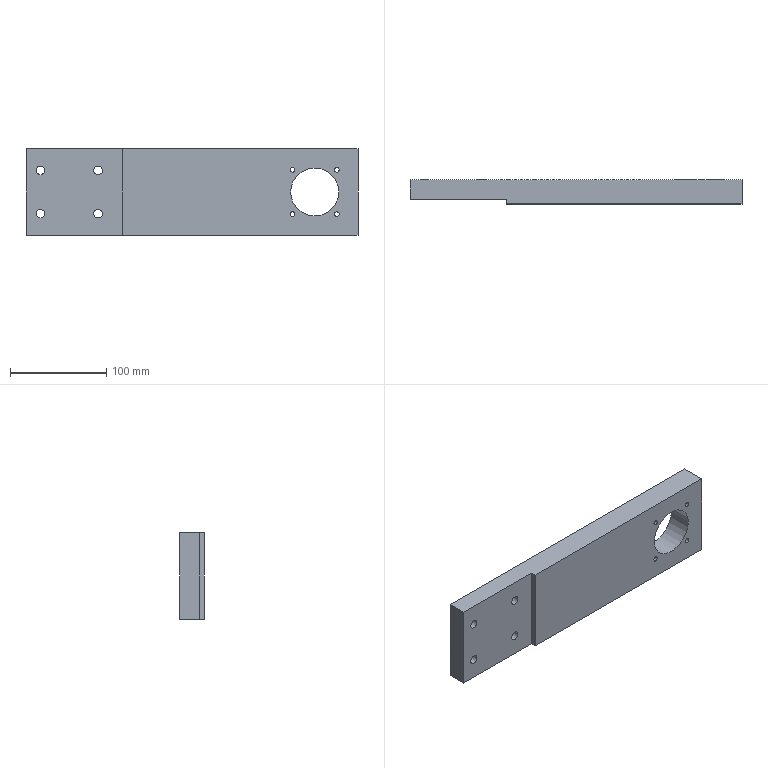Part | STEP file | SN10_001_010_PLACA | 1 solid | 17 faces | box 345 x 25 x 90 mm | volume 675174 mm3 | cylinder 9 | plane 8 | commonest cylinder face diameters 4.917 x4 9 x4 50 x1
STEP:
#1=CARTESIAN_POINT('',(0.,0.,0.));
#2=DIRECTION('',(0.,0.,1.));
#3=DIRECTION('',(1.,0.,0.));
#4=AXIS2_PLACEMENT_3D('',#1,#2,#3);
#5=CARTESIAN_POINT('',(5718.949,200.,24.657));
#6=VERTEX_POINT('',#5);
#7=CARTESIAN_POINT('',(5715.,200.,22.5));
#8=DIRECTION('',(0.,-1.,0.));
#9=DIRECTION('',(1.,0.,0.));
#10=AXIS2_PLACEMENT_3D('',#7,#8,#9);
#11=CIRCLE('',#10,4.5);
#12=CARTESIAN_POINT('',(5715.,199.9,22.5));
#13=DIRECTION('',(0.,-1.,0.));
#14=DIRECTION('',(0.8776,0.,0.4794));
#15=AXIS2_PLACEMENT_3D('',#12,#13,#14);
#16=CYLINDRICAL_SURFACE('',#15,4.5);
#17=CARTESIAN_POINT('',(-0.5,-0.1));
#18=DIRECTION('',(1.,0.));
#19=VECTOR('',#18,1.);
#20=LINE('',#17,#19);
#21=(GEOMETRIC_REPRESENTATION_CONTEXT(2)PARAMETRIC_REPRESENTATION_CONTEXT()REPRESENTATION_CONTEXT('',''));
#22=DEFINITIONAL_REPRESENTATION('',(#20),#21);
#23=PCURVE('',#16,#22);
#24=CARTESIAN_POINT('',(6045.,200.,45.));
#25=DIRECTION('',(0.,-1.,0.));
#26=DIRECTION('',(0.,0.,-1.));
#27=AXIS2_PLACEMENT_3D('',#24,#25,#26);
#28=PLANE('',#27);
#29=CARTESIAN_POINT('',(22.5,-330.));
#30=DIRECTION('',(0.,1.));
#31=AXIS2_PLACEMENT_2D('',#29,#30);
#32=CIRCLE('',#31,4.5);
#33=(GEOMETRIC_REPRESENTATION_CONTEXT(2)PARAMETRIC_REPRESENTATION_CONTEXT()REPRESENTATION_CONTEXT('',''));
#34=DEFINITIONAL_REPRESENTATION('',(#32),#33);
#35=PCURVE('',#28,#34);
#36=SURFACE_CURVE('',#11,(#23,#35),.PCURVE_S1.);
#37=EDGE_CURVE('',#6,#6,#36,.T.);
#38=ORIENTED_EDGE('',*,*,#37,.T.);
#39=CARTESIAN_POINT('',(5718.949,180.,24.657));
#40=VERTEX_POINT('',#39);
#41=CARTESIAN_POINT('',(5718.949,200.,24.657));
#42=CARTESIAN_POINT('',(5718.949,180.,24.657));
#43=B_SPLINE_CURVE_WITH_KNOTS('',1,(#41,#42),.UNSPECIFIED.,.F.,.F.,(2,2),(-0.1,19.9),.PIECEWISE_BEZIER_KNOTS.);
#44=CARTESIAN_POINT('',(6.283,0.));
#45=DIRECTION('',(0.,1.));
#46=VECTOR('',#45,1.);
#47=LINE('',#44,#46);
#48=(GEOMETRIC_REPRESENTATION_CONTEXT(2)PARAMETRIC_REPRESENTATION_CONTEXT()REPRESENTATION_CONTEXT('',''));
#49=DEFINITIONAL_REPRESENTATION('',(#47),#48);
#50=PCURVE('',#16,#49);
#51=CARTESIAN_POINT('',(0.,0.));
#52=DIRECTION('',(0.,1.));
#53=VECTOR('',#52,1.);
#54=LINE('',#51,#53);
#55=(GEOMETRIC_REPRESENTATION_CONTEXT(2)PARAMETRIC_REPRESENTATION_CONTEXT()REPRESENTATION_CONTEXT('',''));
#56=DEFINITIONAL_REPRESENTATION('',(#54),#55);
#57=PCURVE('',#16,#56);
#58=SEAM_CURVE('',#43,(#50,#57),.PCURVE_S1.);
#59=EDGE_CURVE('',#6,#40,#58,.T.);
#60=ORIENTED_EDGE('',*,*,#59,.T.);
#61=CARTESIAN_POINT('',(5715.,180.,22.5));
#62=DIRECTION('',(0.,-1.,0.));
#63=DIRECTION('',(1.,0.,0.));
#64=AXIS2_PLACEMENT_3D('',#61,#62,#63);
#65=CIRCLE('',#64,4.5);
#66=CARTESIAN_POINT('',(-0.5,19.9));
#67=DIRECTION('',(1.,0.));
#68=VECTOR('',#67,1.);
#69=LINE('',#66,#68);
#70=(GEOMETRIC_REPRESENTATION_CONTEXT(2)PARAMETRIC_REPRESENTATION_CONTEXT()REPRESENTATION_CONTEXT('',''));
#71=DEFINITIONAL_REPRESENTATION('',(#69),#70);
#72=PCURVE('',#16,#71);
#73=CARTESIAN_POINT('',(5700.,180.,45.));
#74=DIRECTION('',(0.,1.,0.));
#75=DIRECTION('',(0.,0.,1.));
#76=AXIS2_PLACEMENT_3D('',#73,#74,#75);
#77=PLANE('',#76);
#78=CARTESIAN_POINT('',(-22.5,19.5));
#79=CARTESIAN_POINT('',(-14.706,19.5));
#80=CARTESIAN_POINT('',(-18.603,12.75));
#81=CARTESIAN_POINT('',(-22.5,6.));
#82=CARTESIAN_POINT('',(-26.397,12.75));
#83=CARTESIAN_POINT('',(-30.294,19.5));
#84=CARTESIAN_POINT('',(-22.5,19.5));
#85=(BOUNDED_CURVE()B_SPLINE_CURVE(2,(#78,#79,#80,#81,#82,#83,#84),.UNSPECIFIED.,.T.,.F.)B_SPLINE_CURVE_WITH_KNOTS((1,2,2,2,2,1),(-2.094,0.,2.094,4.189,6.283,8.378),.UNSPECIFIED.)CURVE()GEOMETRIC_REPRESENTATION_ITEM()RATIONAL_B_SPLINE_CURVE((1.,0.5,1.,0.5,1.,0.5,1.))REPRESENTATION_ITEM(''));
#86=(GEOMETRIC_REPRESENTATION_CONTEXT(2)PARAMETRIC_REPRESENTATION_CONTEXT()REPRESENTATION_CONTEXT('',''));
#87=DEFINITIONAL_REPRESENTATION('',(#85),#86);
#88=PCURVE('',#77,#87);
#89=SURFACE_CURVE('',#65,(#72,#88),.PCURVE_S1.);
#90=EDGE_CURVE('',#40,#40,#89,.T.);
#91=ORIENTED_EDGE('',*,*,#90,.F.);
#92=ORIENTED_EDGE('',*,*,#59,.F.);
#93=EDGE_LOOP('',(#38,#60,#91,#92));
#94=FACE_BOUND('',#93,.F.);
#95=ADVANCED_FACE('',(#94),#16,.F.);
#96=CARTESIAN_POINT('',(6045.,175.,-45.));
#97=VERTEX_POINT('',#96);
#98=CARTESIAN_POINT('',(6045.,200.,-45.));
#99=VERTEX_POINT('',#98);
#100=CARTESIAN_POINT('',(6045.,175.,-45.));
#101=DIRECTION('',(0.,1.,0.));
#102=VECTOR('',#101,1.);
#103=LINE('',#100,#102);
#104=CARTESIAN_POINT('',(6045.,175.,45.));
#105=DIRECTION('',(-1.,0.,0.));
#106=DIRECTION('',(0.,0.,1.));
#107=AXIS2_PLACEMENT_3D('',#104,#105,#106);
#108=PLANE('',#107);
#109=CARTESIAN_POINT('',(-90.,0.));
#110=DIRECTION('',(0.,1.));
#111=VECTOR('',#110,1.);
#112=LINE('',#109,#111);
#113=(GEOMETRIC_REPRESENTATION_CONTEXT(2)PARAMETRIC_REPRESENTATION_CONTEXT()REPRESENTATION_CONTEXT('',''));
#114=DEFINITIONAL_REPRESENTATION('',(#112),#113);
#115=PCURVE('',#108,#114);
#116=CARTESIAN_POINT('',(0.,0.,-45.));
#117=DIRECTION('',(0.,0.,1.));
#118=DIRECTION('',(1.,0.,0.));
#119=AXIS2_PLACEMENT_3D('',#116,#117,#118);
#120=PLANE('',#119);
#121=CARTESIAN_POINT('',(6045.,175.));
#122=DIRECTION('',(0.,1.));
#123=VECTOR('',#122,1.);
#124=LINE('',#121,#123);
#125=(GEOMETRIC_REPRESENTATION_CONTEXT(2)PARAMETRIC_REPRESENTATION_CONTEXT()REPRESENTATION_CONTEXT('',''));
#126=DEFINITIONAL_REPRESENTATION('',(#124),#125);
#127=PCURVE('',#120,#126);
#128=SURFACE_CURVE('',#103,(#115,#127),.PCURVE_S1.);
#129=EDGE_CURVE('',#97,#99,#128,.T.);
#130=ORIENTED_EDGE('',*,*,#129,.T.);
#131=CARTESIAN_POINT('',(6045.,200.,45.));
#132=VERTEX_POINT('',#131);
#133=CARTESIAN_POINT('',(6045.,200.,45.));
#134=DIRECTION('',(0.,0.,-1.));
#135=VECTOR('',#134,1.);
#136=LINE('',#133,#135);
#137=CARTESIAN_POINT('',(0.,25.));
#138=DIRECTION('',(-1.,0.));
#139=VECTOR('',#138,1.);
#140=LINE('',#137,#139);
#141=(GEOMETRIC_REPRESENTATION_CONTEXT(2)PARAMETRIC_REPRESENTATION_CONTEXT()REPRESENTATION_CONTEXT('',''));
#142=DEFINITIONAL_REPRESENTATION('',(#140),#141);
#143=PCURVE('',#108,#142);
#144=CARTESIAN_POINT('',(0.,0.));
#145=DIRECTION('',(1.,0.));
#146=VECTOR('',#145,1.);
#147=LINE('',#144,#146);
#148=(GEOMETRIC_REPRESENTATION_CONTEXT(2)PARAMETRIC_REPRESENTATION_CONTEXT()REPRESENTATION_CONTEXT('',''));
#149=DEFINITIONAL_REPRESENTATION('',(#147),#148);
#150=PCURVE('',#28,#149);
#151=SURFACE_CURVE('',#136,(#143,#150),.PCURVE_S1.);
#152=EDGE_CURVE('',#132,#99,#151,.T.);
#153=ORIENTED_EDGE('',*,*,#152,.F.);
#154=CARTESIAN_POINT('',(6045.,175.,45.));
#155=VERTEX_POINT('',#154);
#156=CARTESIAN_POINT('',(6045.,175.,45.));
#157=DIRECTION('',(0.,1.,0.));
#158=VECTOR('',#157,1.);
#159=LINE('',#156,#158);
#160=CARTESIAN_POINT('',(0.,0.));
#161=DIRECTION('',(0.,1.));
#162=VECTOR('',#161,1.);
#163=LINE('',#160,#162);
#164=(GEOMETRIC_REPRESENTATION_CONTEXT(2)PARAMETRIC_REPRESENTATION_CONTEXT()REPRESENTATION_CONTEXT('',''));
#165=DEFINITIONAL_REPRESENTATION('',(#163),#164);
#166=PCURVE('',#108,#165);
#167=CARTESIAN_POINT('',(0.,0.,45.));
#168=DIRECTION('',(0.,0.,1.));
#169=DIRECTION('',(1.,0.,0.));
#170=AXIS2_PLACEMENT_3D('',#167,#168,#169);
#171=PLANE('',#170);
#172=CARTESIAN_POINT('',(6045.,175.));
#173=DIRECTION('',(0.,1.));
#174=VECTOR('',#173,1.);
#175=LINE('',#172,#174);
#176=(GEOMETRIC_REPRESENTATION_CONTEXT(2)PARAMETRIC_REPRESENTATION_CONTEXT()REPRESENTATION_CONTEXT('',''));
#177=DEFINITIONAL_REPRESENTATION('',(#175),#176);
#178=PCURVE('',#171,#177);
#179=SURFACE_CURVE('',#159,(#166,#178),.PCURVE_S1.);
#180=EDGE_CURVE('',#155,#132,#179,.T.);
#181=ORIENTED_EDGE('',*,*,#180,.F.);
#182=CARTESIAN_POINT('',(6045.,175.,45.));
#183=DIRECTION('',(0.,0.,-1.));
#184=VECTOR('',#183,1.);
#185=LINE('',#182,#184);
#186=CARTESIAN_POINT('',(0.,0.));
#187=DIRECTION('',(-1.,0.));
#188=VECTOR('',#187,1.);
#189=LINE('',#186,#188);
#190=(GEOMETRIC_REPRESENTATION_CONTEXT(2)PARAMETRIC_REPRESENTATION_CONTEXT()REPRESENTATION_CONTEXT('',''));
#191=DEFINITIONAL_REPRESENTATION('',(#189),#190);
#192=PCURVE('',#108,#191);
#193=CARTESIAN_POINT('',(5800.,175.,45.));
#194=DIRECTION('',(0.,1.,0.));
#195=DIRECTION('',(0.,0.,1.));
#196=AXIS2_PLACEMENT_3D('',#193,#194,#195);
#197=PLANE('',#196);
#198=CARTESIAN_POINT('',(0.,245.));
#199=DIRECTION('',(-1.,0.));
#200=VECTOR('',#199,1.);
#201=LINE('',#198,#200);
#202=(GEOMETRIC_REPRESENTATION_CONTEXT(2)PARAMETRIC_REPRESENTATION_CONTEXT()REPRESENTATION_CONTEXT('',''));
#203=DEFINITIONAL_REPRESENTATION('',(#201),#202);
#204=PCURVE('',#197,#203);
#205=SURFACE_CURVE('',#185,(#192,#204),.PCURVE_S1.);
#206=EDGE_CURVE('',#155,#97,#205,.T.);
#207=ORIENTED_EDGE('',*,*,#206,.T.);
#208=EDGE_LOOP('',(#130,#153,#181,#207));
#209=FACE_BOUND('',#208,.T.);
#210=ADVANCED_FACE('',(#209),#108,.F.);
#211=CARTESIAN_POINT('',(5700.,200.,-45.));
#212=VERTEX_POINT('',#211);
#213=CARTESIAN_POINT('',(5700.,180.,-45.));
#214=VERTEX_POINT('',#213);
#215=CARTESIAN_POINT('',(5700.,200.,-45.));
#216=DIRECTION('',(0.,-1.,0.));
#217=VECTOR('',#216,1.);
#218=LINE('',#215,#217);
#219=CARTESIAN_POINT('',(5700.,200.));
#220=DIRECTION('',(0.,-1.));
#221=VECTOR('',#220,1.);
#222=LINE('',#219,#221);
#223=(GEOMETRIC_REPRESENTATION_CONTEXT(2)PARAMETRIC_REPRESENTATION_CONTEXT()REPRESENTATION_CONTEXT('',''));
#224=DEFINITIONAL_REPRESENTATION('',(#222),#223);
#225=PCURVE('',#120,#224);
#226=CARTESIAN_POINT('',(5700.,200.,45.));
#227=DIRECTION('',(1.,0.,0.));
#228=DIRECTION('',(0.,0.,-1.));
#229=AXIS2_PLACEMENT_3D('',#226,#227,#228);
#230=PLANE('',#229);
#231=CARTESIAN_POINT('',(90.,0.));
#232=DIRECTION('',(0.,-1.));
#233=VECTOR('',#232,1.);
#234=LINE('',#231,#233);
#235=(GEOMETRIC_REPRESENTATION_CONTEXT(2)PARAMETRIC_REPRESENTATION_CONTEXT()REPRESENTATION_CONTEXT('',''));
#236=DEFINITIONAL_REPRESENTATION('',(#234),#235);
#237=PCURVE('',#230,#236);
#238=SURFACE_CURVE('',#218,(#225,#237),.PCURVE_S1.);
#239=EDGE_CURVE('',#212,#214,#238,.T.);
#240=ORIENTED_EDGE('',*,*,#239,.F.);
#241=CARTESIAN_POINT('',(6045.,200.,-45.));
#242=DIRECTION('',(-1.,0.,0.));
#243=VECTOR('',#242,1.);
#244=LINE('',#241,#243);
#245=CARTESIAN_POINT('',(6045.,200.));
#246=DIRECTION('',(-1.,0.));
#247=VECTOR('',#246,1.);
#248=LINE('',#245,#247);
#249=(GEOMETRIC_REPRESENTATION_CONTEXT(2)PARAMETRIC_REPRESENTATION_CONTEXT()REPRESENTATION_CONTEXT('',''));
#250=DEFINITIONAL_REPRESENTATION('',(#248),#249);
#251=PCURVE('',#120,#250);
#252=CARTESIAN_POINT('',(90.,0.));
#253=DIRECTION('',(0.,-1.));
#254=VECTOR('',#253,1.);
#255=LINE('',#252,#254);
#256=(GEOMETRIC_REPRESENTATION_CONTEXT(2)PARAMETRIC_REPRESENTATION_CONTEXT()REPRESENTATION_CONTEXT('',''));
#257=DEFINITIONAL_REPRESENTATION('',(#255),#256);
#258=PCURVE('',#28,#257);
#259=SURFACE_CURVE('',#244,(#251,#258),.PCURVE_S1.);
#260=EDGE_CURVE('',#99,#212,#259,.T.);
#261=ORIENTED_EDGE('',*,*,#260,.F.);
#262=ORIENTED_EDGE('',*,*,#129,.F.);
#263=CARTESIAN_POINT('',(5800.,175.,-45.));
#264=VERTEX_POINT('',#263);
#265=CARTESIAN_POINT('',(5800.,175.,-45.));
#266=DIRECTION('',(1.,0.,0.));
#267=VECTOR('',#266,1.);
#268=LINE('',#265,#267);
#269=CARTESIAN_POINT('',(5800.,175.));
#270=DIRECTION('',(1.,0.));
#271=VECTOR('',#270,1.);
#272=LINE('',#269,#271);
#273=(GEOMETRIC_REPRESENTATION_CONTEXT(2)PARAMETRIC_REPRESENTATION_CONTEXT()REPRESENTATION_CONTEXT('',''));
#274=DEFINITIONAL_REPRESENTATION('',(#272),#273);
#275=PCURVE('',#120,#274);
#276=CARTESIAN_POINT('',(-90.,0.));
#277=DIRECTION('',(0.,1.));
#278=VECTOR('',#277,1.);
#279=LINE('',#276,#278);
#280=(GEOMETRIC_REPRESENTATION_CONTEXT(2)PARAMETRIC_REPRESENTATION_CONTEXT()REPRESENTATION_CONTEXT('',''));
#281=DEFINITIONAL_REPRESENTATION('',(#279),#280);
#282=PCURVE('',#197,#281);
#283=SURFACE_CURVE('',#268,(#275,#282),.PCURVE_S1.);
#284=EDGE_CURVE('',#264,#97,#283,.T.);
#285=ORIENTED_EDGE('',*,*,#284,.F.);
#286=CARTESIAN_POINT('',(5800.,180.,-45.));
#287=VERTEX_POINT('',#286);
#288=CARTESIAN_POINT('',(5800.,180.,-45.));
#289=DIRECTION('',(0.,-1.,0.));
#290=VECTOR('',#289,1.);
#291=LINE('',#288,#290);
#292=CARTESIAN_POINT('',(5800.,180.));
#293=DIRECTION('',(0.,-1.));
#294=VECTOR('',#293,1.);
#295=LINE('',#292,#294);
#296=(GEOMETRIC_REPRESENTATION_CONTEXT(2)PARAMETRIC_REPRESENTATION_CONTEXT()REPRESENTATION_CONTEXT('',''));
#297=DEFINITIONAL_REPRESENTATION('',(#295),#296);
#298=PCURVE('',#120,#297);
#299=CARTESIAN_POINT('',(5800.,180.,45.));
#300=DIRECTION('',(1.,0.,0.));
#301=DIRECTION('',(0.,0.,-1.));
#302=AXIS2_PLACEMENT_3D('',#299,#300,#301);
#303=PLANE('',#302);
#304=CARTESIAN_POINT('',(90.,0.));
#305=DIRECTION('',(0.,-1.));
#306=VECTOR('',#305,1.);
#307=LINE('',#304,#306);
#308=(GEOMETRIC_REPRESENTATION_CONTEXT(2)PARAMETRIC_REPRESENTATION_CONTEXT()REPRESENTATION_CONTEXT('',''));
#309=DEFINITIONAL_REPRESENTATION('',(#307),#308);
#310=PCURVE('',#303,#309);
#311=SURFACE_CURVE('',#291,(#298,#310),.PCURVE_S1.);
#312=EDGE_CURVE('',#287,#264,#311,.T.);
#313=ORIENTED_EDGE('',*,*,#312,.F.);
#314=CARTESIAN_POINT('',(5700.,180.,-45.));
#315=DIRECTION('',(1.,0.,0.));
#316=VECTOR('',#315,1.);
#317=LINE('',#314,#316);
#318=CARTESIAN_POINT('',(5700.,180.));
#319=DIRECTION('',(1.,0.));
#320=VECTOR('',#319,1.);
#321=LINE('',#318,#320);
#322=(GEOMETRIC_REPRESENTATION_CONTEXT(2)PARAMETRIC_REPRESENTATION_CONTEXT()REPRESENTATION_CONTEXT('',''));
#323=DEFINITIONAL_REPRESENTATION('',(#321),#322);
#324=PCURVE('',#120,#323);
#325=CARTESIAN_POINT('',(-90.,0.));
#326=DIRECTION('',(0.,1.));
#327=VECTOR('',#326,1.);
#328=LINE('',#325,#327);
#329=(GEOMETRIC_REPRESENTATION_CONTEXT(2)PARAMETRIC_REPRESENTATION_CONTEXT()REPRESENTATION_CONTEXT('',''));
#330=DEFINITIONAL_REPRESENTATION('',(#328),#329);
#331=PCURVE('',#77,#330);
#332=SURFACE_CURVE('',#317,(#324,#331),.PCURVE_S1.);
#333=EDGE_CURVE('',#214,#287,#332,.T.);
#334=ORIENTED_EDGE('',*,*,#333,.F.);
#335=EDGE_LOOP('',(#240,#261,#262,#285,#313,#334));
#336=FACE_BOUND('',#335,.T.);
#337=ADVANCED_FACE('',(#336),#120,.F.);
#338=CARTESIAN_POINT('',(6020.823,200.,21.802));
#339=VERTEX_POINT('',#338);
#340=CARTESIAN_POINT('',(6022.981,200.,22.981));
#341=DIRECTION('',(0.,-1.,0.));
#342=DIRECTION('',(1.,0.,0.));
#343=AXIS2_PLACEMENT_3D('',#340,#341,#342);
#344=CIRCLE('',#343,2.458);
#345=CARTESIAN_POINT('',(6022.981,199.9,22.981));
#346=DIRECTION('',(0.,-1.,0.));
#347=DIRECTION('',(0.8776,0.,0.4794));
#348=AXIS2_PLACEMENT_3D('',#345,#346,#347);
#349=CYLINDRICAL_SURFACE('',#348,2.458);
#350=CARTESIAN_POINT('',(-0.5,-0.1));
#351=DIRECTION('',(1.,0.));
#352=VECTOR('',#351,1.);
#353=LINE('',#350,#352);
#354=(GEOMETRIC_REPRESENTATION_CONTEXT(2)PARAMETRIC_REPRESENTATION_CONTEXT()REPRESENTATION_CONTEXT('',''));
#355=DEFINITIONAL_REPRESENTATION('',(#353),#354);
#356=PCURVE('',#349,#355);
#357=CARTESIAN_POINT('',(22.019,-22.019));
#358=DIRECTION('',(0.,1.));
#359=AXIS2_PLACEMENT_2D('',#357,#358);
#360=CIRCLE('',#359,2.458);
#361=(GEOMETRIC_REPRESENTATION_CONTEXT(2)PARAMETRIC_REPRESENTATION_CONTEXT()REPRESENTATION_CONTEXT('',''));
#362=DEFINITIONAL_REPRESENTATION('',(#360),#361);
#363=PCURVE('',#28,#362);
#364=SURFACE_CURVE('',#344,(#356,#363),.PCURVE_S1.);
#365=EDGE_CURVE('',#339,#339,#364,.T.);
#366=ORIENTED_EDGE('',*,*,#365,.T.);
#367=CARTESIAN_POINT('',(6020.823,175.,21.802));
#368=VERTEX_POINT('',#367);
#369=CARTESIAN_POINT('',(6020.823,200.,21.802));
#370=CARTESIAN_POINT('',(6020.823,175.,21.802));
#371=B_SPLINE_CURVE_WITH_KNOTS('',1,(#369,#370),.UNSPECIFIED.,.F.,.F.,(2,2),(-0.1,24.9),.PIECEWISE_BEZIER_KNOTS.);
#372=CARTESIAN_POINT('',(9.425,0.));
#373=DIRECTION('',(0.,1.));
#374=VECTOR('',#373,1.);
#375=LINE('',#372,#374);
#376=(GEOMETRIC_REPRESENTATION_CONTEXT(2)PARAMETRIC_REPRESENTATION_CONTEXT()REPRESENTATION_CONTEXT('',''));
#377=DEFINITIONAL_REPRESENTATION('',(#375),#376);
#378=PCURVE('',#349,#377);
#379=CARTESIAN_POINT('',(3.142,0.));
#380=DIRECTION('',(0.,1.));
#381=VECTOR('',#380,1.);
#382=LINE('',#379,#381);
#383=(GEOMETRIC_REPRESENTATION_CONTEXT(2)PARAMETRIC_REPRESENTATION_CONTEXT()REPRESENTATION_CONTEXT('',''));
#384=DEFINITIONAL_REPRESENTATION('',(#382),#383);
#385=PCURVE('',#349,#384);
#386=SEAM_CURVE('',#371,(#378,#385),.PCURVE_S1.);
#387=EDGE_CURVE('',#339,#368,#386,.T.);
#388=ORIENTED_EDGE('',*,*,#387,.T.);
#389=CARTESIAN_POINT('',(6022.981,175.,22.981));
#390=DIRECTION('',(0.,-1.,0.));
#391=DIRECTION('',(1.,0.,0.));
#392=AXIS2_PLACEMENT_3D('',#389,#390,#391);
#393=CIRCLE('',#392,2.458);
#394=CARTESIAN_POINT('',(-0.5,24.9));
#395=DIRECTION('',(1.,0.));
#396=VECTOR('',#395,1.);
#397=LINE('',#394,#396);
#398=(GEOMETRIC_REPRESENTATION_CONTEXT(2)PARAMETRIC_REPRESENTATION_CONTEXT()REPRESENTATION_CONTEXT('',''));
#399=DEFINITIONAL_REPRESENTATION('',(#397),#398);
#400=PCURVE('',#349,#399);
#401=CARTESIAN_POINT('',(-22.019,225.439));
#402=CARTESIAN_POINT('',(-17.761,225.439));
#403=CARTESIAN_POINT('',(-19.89,221.752));
#404=CARTESIAN_POINT('',(-22.019,218.064));
#405=CARTESIAN_POINT('',(-24.148,221.752));
#406=CARTESIAN_POINT('',(-26.277,225.439));
#407=CARTESIAN_POINT('',(-22.019,225.439));
#408=(BOUNDED_CURVE()B_SPLINE_CURVE(2,(#401,#402,#403,#404,#405,#406,#407),.UNSPECIFIED.,.T.,.F.)B_SPLINE_CURVE_WITH_KNOTS((1,2,2,2,2,1),(-2.094,0.,2.094,4.189,6.283,8.378),.UNSPECIFIED.)CURVE()GEOMETRIC_REPRESENTATION_ITEM()RATIONAL_B_SPLINE_CURVE((1.,0.5,1.,0.5,1.,0.5,1.))REPRESENTATION_ITEM(''));
#409=(GEOMETRIC_REPRESENTATION_CONTEXT(2)PARAMETRIC_REPRESENTATION_CONTEXT()REPRESENTATION_CONTEXT('',''));
#410=DEFINITIONAL_REPRESENTATION('',(#408),#409);
#411=PCURVE('',#197,#410);
#412=SURFACE_CURVE('',#393,(#400,#411),.PCURVE_S1.);
#413=EDGE_CURVE('',#368,#368,#412,.T.);
#414=ORIENTED_EDGE('',*,*,#413,.F.);
#415=ORIENTED_EDGE('',*,*,#387,.F.);
#416=EDGE_LOOP('',(#366,#388,#414,#415));
#417=FACE_BOUND('',#416,.F.);
#418=ADVANCED_FACE('',(#417),#349,.F.);
#419=CARTESIAN_POINT('',(5975.,200.,0.));
#420=VERTEX_POINT('',#419);
#421=CARTESIAN_POINT('',(6000.,200.,0.));
#422=DIRECTION('',(0.,-1.,0.));
#423=DIRECTION('',(1.,0.,0.));
#424=AXIS2_PLACEMENT_3D('',#421,#422,#423);
#425=CIRCLE('',#424,25.);
#426=CARTESIAN_POINT('',(6000.,188.16,0.));
#427=DIRECTION('',(0.,-1.,0.));
#428=DIRECTION('',(1.,0.,0.));
#429=AXIS2_PLACEMENT_3D('',#426,#427,#428);
#430=CYLINDRICAL_SURFACE('',#429,25.);
#431=CARTESIAN_POINT('',(0.,-11.84));
#432=DIRECTION('',(1.,0.));
#433=VECTOR('',#432,1.);
#434=LINE('',#431,#433);
#435=(GEOMETRIC_REPRESENTATION_CONTEXT(2)PARAMETRIC_REPRESENTATION_CONTEXT()REPRESENTATION_CONTEXT('',''));
#436=DEFINITIONAL_REPRESENTATION('',(#434),#435);
#437=PCURVE('',#430,#436);
#438=CARTESIAN_POINT('',(45.,-45.));
#439=DIRECTION('',(0.,1.));
#440=AXIS2_PLACEMENT_2D('',#438,#439);
#441=CIRCLE('',#440,25.);
#442=(GEOMETRIC_REPRESENTATION_CONTEXT(2)PARAMETRIC_REPRESENTATION_CONTEXT()REPRESENTATION_CONTEXT('',''));
#443=DEFINITIONAL_REPRESENTATION('',(#441),#442);
#444=PCURVE('',#28,#443);
#445=SURFACE_CURVE('',#425,(#437,#444),.PCURVE_S1.);
#446=EDGE_CURVE('',#420,#420,#445,.T.);
#447=ORIENTED_EDGE('',*,*,#446,.T.);
#448=CARTESIAN_POINT('',(5975.,175.,0.));
#449=VERTEX_POINT('',#448);
#450=CARTESIAN_POINT('',(5975.,200.,0.));
#451=CARTESIAN_POINT('',(5975.,175.,0.));
#452=B_SPLINE_CURVE_WITH_KNOTS('',1,(#450,#451),.UNSPECIFIED.,.F.,.F.,(2,2),(-11.84,13.16),.PIECEWISE_BEZIER_KNOTS.);
#453=CARTESIAN_POINT('',(9.425,0.));
#454=DIRECTION('',(0.,1.));
#455=VECTOR('',#454,1.);
#456=LINE('',#453,#455);
#457=(GEOMETRIC_REPRESENTATION_CONTEXT(2)PARAMETRIC_REPRESENTATION_CONTEXT()REPRESENTATION_CONTEXT('',''));
#458=DEFINITIONAL_REPRESENTATION('',(#456),#457);
#459=PCURVE('',#430,#458);
#460=CARTESIAN_POINT('',(3.142,0.));
#461=DIRECTION('',(0.,1.));
#462=VECTOR('',#461,1.);
#463=LINE('',#460,#462);
#464=(GEOMETRIC_REPRESENTATION_CONTEXT(2)PARAMETRIC_REPRESENTATION_CONTEXT()REPRESENTATION_CONTEXT('',''));
#465=DEFINITIONAL_REPRESENTATION('',(#463),#464);
#466=PCURVE('',#430,#465);
#467=SEAM_CURVE('',#452,(#459,#466),.PCURVE_S1.);
#468=EDGE_CURVE('',#420,#449,#467,.T.);
#469=ORIENTED_EDGE('',*,*,#468,.T.);
#470=CARTESIAN_POINT('',(6000.,175.,0.));
#471=DIRECTION('',(0.,-1.,0.));
#472=DIRECTION('',(1.,0.,0.));
#473=AXIS2_PLACEMENT_3D('',#470,#471,#472);
#474=CIRCLE('',#473,25.);
#475=CARTESIAN_POINT('',(0.,13.16));
#476=DIRECTION('',(1.,0.));
#477=VECTOR('',#476,1.);
#478=LINE('',#475,#477);
#479=(GEOMETRIC_REPRESENTATION_CONTEXT(2)PARAMETRIC_REPRESENTATION_CONTEXT()REPRESENTATION_CONTEXT('',''));
#480=DEFINITIONAL_REPRESENTATION('',(#478),#479);
#481=PCURVE('',#430,#480);
#482=CARTESIAN_POINT('',(-45.,225.));
#483=CARTESIAN_POINT('',(-1.699,225.));
#484=CARTESIAN_POINT('',(-23.349,187.5));
#485=CARTESIAN_POINT('',(-45.,150.));
#486=CARTESIAN_POINT('',(-66.651,187.5));
#487=CARTESIAN_POINT('',(-88.301,225.));
#488=CARTESIAN_POINT('',(-45.,225.));
#489=(BOUNDED_CURVE()B_SPLINE_CURVE(2,(#482,#483,#484,#485,#486,#487,#488),.UNSPECIFIED.,.T.,.F.)B_SPLINE_CURVE_WITH_KNOTS((1,2,2,2,2,1),(-2.094,0.,2.094,4.189,6.283,8.378),.UNSPECIFIED.)CURVE()GEOMETRIC_REPRESENTATION_ITEM()RATIONAL_B_SPLINE_CURVE((1.,0.5,1.,0.5,1.,0.5,1.))REPRESENTATION_ITEM(''));
#490=(GEOMETRIC_REPRESENTATION_CONTEXT(2)PARAMETRIC_REPRESENTATION_CONTEXT()REPRESENTATION_CONTEXT('',''));
#491=DEFINITIONAL_REPRESENTATION('',(#489),#490);
#492=PCURVE('',#197,#491);
#493=SURFACE_CURVE('',#474,(#481,#492),.PCURVE_S1.);
#494=EDGE_CURVE('',#449,#449,#493,.T.);
#495=ORIENTED_EDGE('',*,*,#494,.F.);
#496=ORIENTED_EDGE('',*,*,#468,.F.);
#497=EDGE_LOOP('',(#447,#469,#495,#496));
#498=FACE_BOUND('',#497,.F.);
#499=ADVANCED_FACE('',(#498),#430,.F.);
#500=CARTESIAN_POINT('',(6024.16,200.,-25.139));
#501=VERTEX_POINT('',#500);
#502=CARTESIAN_POINT('',(6022.981,200.,-22.981));
#503=DIRECTION('',(0.,-1.,0.));
#504=DIRECTION('',(1.,0.,0.));
#505=AXIS2_PLACEMENT_3D('',#502,#503,#504);
#506=CIRCLE('',#505,2.458);
#507=CARTESIAN_POINT('',(6022.981,199.9,-22.981));
#508=DIRECTION('',(0.,-1.,0.));
#509=DIRECTION('',(0.4794,0.,-0.8776));
#510=AXIS2_PLACEMENT_3D('',#507,#508,#509);
#511=CYLINDRICAL_SURFACE('',#510,2.458);
#512=CARTESIAN_POINT('',(1.071,-0.1));
#513=DIRECTION('',(1.,0.));
#514=VECTOR('',#513,1.);
#515=LINE('',#512,#514);
#516=(GEOMETRIC_REPRESENTATION_CONTEXT(2)PARAMETRIC_REPRESENTATION_CONTEXT()REPRESENTATION_CONTEXT('',''));
#517=DEFINITIONAL_REPRESENTATION('',(#515),#516);
#518=PCURVE('',#511,#517);
#519=CARTESIAN_POINT('',(67.981,-22.019));
#520=DIRECTION('',(0.,1.));
#521=AXIS2_PLACEMENT_2D('',#519,#520);
#522=CIRCLE('',#521,2.458);
#523=(GEOMETRIC_REPRESENTATION_CONTEXT(2)PARAMETRIC_REPRESENTATION_CONTEXT()REPRESENTATION_CONTEXT('',''));
#524=DEFINITIONAL_REPRESENTATION('',(#522),#523);
#525=PCURVE('',#28,#524);
#526=SURFACE_CURVE('',#506,(#518,#525),.PCURVE_S1.);
#527=EDGE_CURVE('',#501,#501,#526,.T.);
#528=ORIENTED_EDGE('',*,*,#527,.T.);
#529=CARTESIAN_POINT('',(6024.16,175.,-25.139));
#530=VERTEX_POINT('',#529);
#531=CARTESIAN_POINT('',(6024.16,200.,-25.139));
#532=CARTESIAN_POINT('',(6024.16,175.,-25.139));
#533=B_SPLINE_CURVE_WITH_KNOTS('',1,(#531,#532),.UNSPECIFIED.,.F.,.F.,(2,2),(-0.1,24.9),.PIECEWISE_BEZIER_KNOTS.);
#534=CARTESIAN_POINT('',(12.566,0.));
#535=DIRECTION('',(0.,1.));
#536=VECTOR('',#535,1.);
#537=LINE('',#534,#536);
#538=(GEOMETRIC_REPRESENTATION_CONTEXT(2)PARAMETRIC_REPRESENTATION_CONTEXT()REPRESENTATION_CONTEXT('',''));
#539=DEFINITIONAL_REPRESENTATION('',(#537),#538);
#540=PCURVE('',#511,#539);
#541=CARTESIAN_POINT('',(6.283,0.));
#542=DIRECTION('',(0.,1.));
#543=VECTOR('',#542,1.);
#544=LINE('',#541,#543);
#545=(GEOMETRIC_REPRESENTATION_CONTEXT(2)PARAMETRIC_REPRESENTATION_CONTEXT()REPRESENTATION_CONTEXT('',''));
#546=DEFINITIONAL_REPRESENTATION('',(#544),#545);
#547=PCURVE('',#511,#546);
#548=SEAM_CURVE('',#533,(#540,#547),.PCURVE_S1.);
#549=EDGE_CURVE('',#501,#530,#548,.T.);
#550=ORIENTED_EDGE('',*,*,#549,.T.);
#551=CARTESIAN_POINT('',(6022.981,175.,-22.981));
#552=DIRECTION('',(0.,-1.,0.));
#553=DIRECTION('',(1.,0.,0.));
#554=AXIS2_PLACEMENT_3D('',#551,#552,#553);
#555=CIRCLE('',#554,2.458);
#556=CARTESIAN_POINT('',(1.071,24.9));
#557=DIRECTION('',(1.,0.));
#558=VECTOR('',#557,1.);
#559=LINE('',#556,#558);
#560=(GEOMETRIC_REPRESENTATION_CONTEXT(2)PARAMETRIC_REPRESENTATION_CONTEXT()REPRESENTATION_CONTEXT('',''));
#561=DEFINITIONAL_REPRESENTATION('',(#559),#560);
#562=PCURVE('',#511,#561);
#563=CARTESIAN_POINT('',(-67.981,225.439));
#564=CARTESIAN_POINT('',(-63.723,225.439));
#565=CARTESIAN_POINT('',(-65.852,221.752));
#566=CARTESIAN_POINT('',(-67.981,218.064));
#567=CARTESIAN_POINT('',(-70.11,221.752));
#568=CARTESIAN_POINT('',(-72.239,225.439));
#569=CARTESIAN_POINT('',(-67.981,225.439));
#570=(BOUNDED_CURVE()B_SPLINE_CURVE(2,(#563,#564,#565,#566,#567,#568,#569),.UNSPECIFIED.,.T.,.F.)B_SPLINE_CURVE_WITH_KNOTS((1,2,2,2,2,1),(-2.094,0.,2.094,4.189,6.283,8.378),.UNSPECIFIED.)CURVE()GEOMETRIC_REPRESENTATION_ITEM()RATIONAL_B_SPLINE_CURVE((1.,0.5,1.,0.5,1.,0.5,1.))REPRESENTATION_ITEM(''));
#571=(GEOMETRIC_REPRESENTATION_CONTEXT(2)PARAMETRIC_REPRESENTATION_CONTEXT()REPRESENTATION_CONTEXT('',''));
#572=DEFINITIONAL_REPRESENTATION('',(#570),#571);
#573=PCURVE('',#197,#572);
#574=SURFACE_CURVE('',#555,(#562,#573),.PCURVE_S1.);
#575=EDGE_CURVE('',#530,#530,#574,.T.);
#576=ORIENTED_EDGE('',*,*,#575,.F.);
#577=ORIENTED_EDGE('',*,*,#549,.F.);
#578=EDGE_LOOP('',(#528,#550,#576,#577));
#579=FACE_BOUND('',#578,.F.);
#580=ADVANCED_FACE('',(#579),#511,.F.);
#581=CARTESIAN_POINT('',(5974.861,200.,-24.16));
#582=VERTEX_POINT('',#581);
#583=CARTESIAN_POINT('',(5977.019,200.,-22.981));
#584=DIRECTION('',(0.,-1.,0.));
#585=DIRECTION('',(1.,0.,0.));
#586=AXIS2_PLACEMENT_3D('',#583,#584,#585);
#587=CIRCLE('',#586,2.458);
#588=CARTESIAN_POINT('',(5977.019,199.9,-22.981));
#589=DIRECTION('',(0.,-1.,0.));
#590=DIRECTION('',(-0.8776,0.,-0.4794));
#591=AXIS2_PLACEMENT_3D('',#588,#589,#590);
#592=CYLINDRICAL_SURFACE('',#591,2.458);
#593=CARTESIAN_POINT('',(-3.642,-0.1));
#594=DIRECTION('',(1.,0.));
#595=VECTOR('',#594,1.);
#596=LINE('',#593,#595);
#597=(GEOMETRIC_REPRESENTATION_CONTEXT(2)PARAMETRIC_REPRESENTATION_CONTEXT()REPRESENTATION_CONTEXT('',''));
#598=DEFINITIONAL_REPRESENTATION('',(#596),#597);
#599=PCURVE('',#592,#598);
#600=CARTESIAN_POINT('',(67.981,-67.981));
#601=DIRECTION('',(0.,1.));
#602=AXIS2_PLACEMENT_2D('',#600,#601);
#603=CIRCLE('',#602,2.458);
#604=(GEOMETRIC_REPRESENTATION_CONTEXT(2)PARAMETRIC_REPRESENTATION_CONTEXT()REPRESENTATION_CONTEXT('',''));
#605=DEFINITIONAL_REPRESENTATION('',(#603),#604);
#606=PCURVE('',#28,#605);
#607=SURFACE_CURVE('',#587,(#599,#606),.PCURVE_S1.);
#608=EDGE_CURVE('',#582,#582,#607,.T.);
#609=ORIENTED_EDGE('',*,*,#608,.T.);
#610=CARTESIAN_POINT('',(5974.861,175.,-24.16));
#611=VERTEX_POINT('',#610);
#612=CARTESIAN_POINT('',(5974.861,200.,-24.16));
#613=CARTESIAN_POINT('',(5974.861,175.,-24.16));
#614=B_SPLINE_CURVE_WITH_KNOTS('',1,(#612,#613),.UNSPECIFIED.,.F.,.F.,(2,2),(-0.1,24.9),.PIECEWISE_BEZIER_KNOTS.);
#615=CARTESIAN_POINT('',(6.283,0.));
#616=DIRECTION('',(0.,1.));
#617=VECTOR('',#616,1.);
#618=LINE('',#615,#617);
#619=(GEOMETRIC_REPRESENTATION_CONTEXT(2)PARAMETRIC_REPRESENTATION_CONTEXT()REPRESENTATION_CONTEXT('',''));
#620=DEFINITIONAL_REPRESENTATION('',(#618),#619);
#621=PCURVE('',#592,#620);
#622=CARTESIAN_POINT('',(0.,0.));
#623=DIRECTION('',(0.,1.));
#624=VECTOR('',#623,1.);
#625=LINE('',#622,#624);
#626=(GEOMETRIC_REPRESENTATION_CONTEXT(2)PARAMETRIC_REPRESENTATION_CONTEXT()REPRESENTATION_CONTEXT('',''));
#627=DEFINITIONAL_REPRESENTATION('',(#625),#626);
#628=PCURVE('',#592,#627);
#629=SEAM_CURVE('',#614,(#621,#628),.PCURVE_S1.);
#630=EDGE_CURVE('',#582,#611,#629,.T.);
#631=ORIENTED_EDGE('',*,*,#630,.T.);
#632=CARTESIAN_POINT('',(5977.019,175.,-22.981));
#633=DIRECTION('',(0.,-1.,0.));
#634=DIRECTION('',(1.,0.,0.));
#635=AXIS2_PLACEMENT_3D('',#632,#633,#634);
#636=CIRCLE('',#635,2.458);
#637=CARTESIAN_POINT('',(-3.642,24.9));
#638=DIRECTION('',(1.,0.));
#639=VECTOR('',#638,1.);
#640=LINE('',#637,#639);
#641=(GEOMETRIC_REPRESENTATION_CONTEXT(2)PARAMETRIC_REPRESENTATION_CONTEXT()REPRESENTATION_CONTEXT('',''));
#642=DEFINITIONAL_REPRESENTATION('',(#640),#641);
#643=PCURVE('',#592,#642);
#644=CARTESIAN_POINT('',(-67.981,179.478));
#645=CARTESIAN_POINT('',(-63.723,179.478));
#646=CARTESIAN_POINT('',(-65.852,175.79));
#647=CARTESIAN_POINT('',(-67.981,172.102));
#648=CARTESIAN_POINT('',(-70.11,175.79));
#649=CARTESIAN_POINT('',(-72.239,179.478));
#650=CARTESIAN_POINT('',(-67.981,179.478));
#651=(BOUNDED_CURVE()B_SPLINE_CURVE(2,(#644,#645,#646,#647,#648,#649,#650),.UNSPECIFIED.,.T.,.F.)B_SPLINE_CURVE_WITH_KNOTS((1,2,2,2,2,1),(-2.094,0.,2.094,4.189,6.283,8.378),.UNSPECIFIED.)CURVE()GEOMETRIC_REPRESENTATION_ITEM()RATIONAL_B_SPLINE_CURVE((1.,0.5,1.,0.5,1.,0.5,1.))REPRESENTATION_ITEM(''));
#652=(GEOMETRIC_REPRESENTATION_CONTEXT(2)PARAMETRIC_REPRESENTATION_CONTEXT()REPRESENTATION_CONTEXT('',''));
#653=DEFINITIONAL_REPRESENTATION('',(#651),#652);
#654=PCURVE('',#197,#653);
#655=SURFACE_CURVE('',#636,(#643,#654),.PCURVE_S1.);
#656=EDGE_CURVE('',#611,#611,#655,.T.);
#657=ORIENTED_EDGE('',*,*,#656,.F.);
#658=ORIENTED_EDGE('',*,*,#630,.F.);
#659=EDGE_LOOP('',(#609,#631,#657,#658));
#660=FACE_BOUND('',#659,.F.);
#661=ADVANCED_FACE('',(#660),#592,.F.);
#662=CARTESIAN_POINT('',(5975.84,200.,25.139));
#663=VERTEX_POINT('',#662);
#664=CARTESIAN_POINT('',(5977.019,200.,22.981));
#665=DIRECTION('',(0.,-1.,0.));
#666=DIRECTION('',(1.,0.,0.));
#667=AXIS2_PLACEMENT_3D('',#664,#665,#666);
#668=CIRCLE('',#667,2.458);
#669=CARTESIAN_POINT('',(5977.019,199.9,22.981));
#670=DIRECTION('',(0.,-1.,0.));
#671=DIRECTION('',(-0.4794,0.,0.8776));
#672=AXIS2_PLACEMENT_3D('',#669,#670,#671);
#673=CYLINDRICAL_SURFACE('',#672,2.458);
#674=CARTESIAN_POINT('',(-2.071,-0.1));
#675=DIRECTION('',(1.,0.));
#676=VECTOR('',#675,1.);
#677=LINE('',#674,#676);
#678=(GEOMETRIC_REPRESENTATION_CONTEXT(2)PARAMETRIC_REPRESENTATION_CONTEXT()REPRESENTATION_CONTEXT('',''));
#679=DEFINITIONAL_REPRESENTATION('',(#677),#678);
#680=PCURVE('',#673,#679);
#681=CARTESIAN_POINT('',(22.019,-67.981));
#682=DIRECTION('',(0.,1.));
#683=AXIS2_PLACEMENT_2D('',#681,#682);
#684=CIRCLE('',#683,2.458);
#685=(GEOMETRIC_REPRESENTATION_CONTEXT(2)PARAMETRIC_REPRESENTATION_CONTEXT()REPRESENTATION_CONTEXT('',''));
#686=DEFINITIONAL_REPRESENTATION('',(#684),#685);
#687=PCURVE('',#28,#686);
#688=SURFACE_CURVE('',#668,(#680,#687),.PCURVE_S1.);
#689=EDGE_CURVE('',#663,#663,#688,.T.);
#690=ORIENTED_EDGE('',*,*,#689,.T.);
#691=CARTESIAN_POINT('',(5975.84,175.,25.139));
#692=VERTEX_POINT('',#691);
#693=CARTESIAN_POINT('',(5975.84,200.,25.139));
#694=CARTESIAN_POINT('',(5975.84,175.,25.139));
#695=B_SPLINE_CURVE_WITH_KNOTS('',1,(#693,#694),.UNSPECIFIED.,.F.,.F.,(2,2),(-0.1,24.9),.PIECEWISE_BEZIER_KNOTS.);
#696=CARTESIAN_POINT('',(6.283,0.));
#697=DIRECTION('',(0.,1.));
#698=VECTOR('',#697,1.);
#699=LINE('',#696,#698);
#700=(GEOMETRIC_REPRESENTATION_CONTEXT(2)PARAMETRIC_REPRESENTATION_CONTEXT()REPRESENTATION_CONTEXT('',''));
#701=DEFINITIONAL_REPRESENTATION('',(#699),#700);
#702=PCURVE('',#673,#701);
#703=CARTESIAN_POINT('',(0.,0.));
#704=DIRECTION('',(0.,1.));
#705=VECTOR('',#704,1.);
#706=LINE('',#703,#705);
#707=(GEOMETRIC_REPRESENTATION_CONTEXT(2)PARAMETRIC_REPRESENTATION_CONTEXT()REPRESENTATION_CONTEXT('',''));
#708=DEFINITIONAL_REPRESENTATION('',(#706),#707);
#709=PCURVE('',#673,#708);
#710=SEAM_CURVE('',#695,(#702,#709),.PCURVE_S1.);
#711=EDGE_CURVE('',#663,#692,#710,.T.);
#712=ORIENTED_EDGE('',*,*,#711,.T.);
#713=CARTESIAN_POINT('',(5977.019,175.,22.981));
#714=DIRECTION('',(0.,-1.,0.));
#715=DIRECTION('',(1.,0.,0.));
#716=AXIS2_PLACEMENT_3D('',#713,#714,#715);
#717=CIRCLE('',#716,2.458);
#718=CARTESIAN_POINT('',(-2.071,24.9));
#719=DIRECTION('',(1.,0.));
#720=VECTOR('',#719,1.);
#721=LINE('',#718,#720);
#722=(GEOMETRIC_REPRESENTATION_CONTEXT(2)PARAMETRIC_REPRESENTATION_CONTEXT()REPRESENTATION_CONTEXT('',''));
#723=DEFINITIONAL_REPRESENTATION('',(#721),#722);
#724=PCURVE('',#673,#723);
#725=CARTESIAN_POINT('',(-22.019,179.478));
#726=CARTESIAN_POINT('',(-17.761,179.478));
#727=CARTESIAN_POINT('',(-19.89,175.79));
#728=CARTESIAN_POINT('',(-22.019,172.102));
#729=CARTESIAN_POINT('',(-24.148,175.79));
#730=CARTESIAN_POINT('',(-26.277,179.478));
#731=CARTESIAN_POINT('',(-22.019,179.478));
#732=(BOUNDED_CURVE()B_SPLINE_CURVE(2,(#725,#726,#727,#728,#729,#730,#731),.UNSPECIFIED.,.T.,.F.)B_SPLINE_CURVE_WITH_KNOTS((1,2,2,2,2,1),(-2.094,0.,2.094,4.189,6.283,8.378),.UNSPECIFIED.)CURVE()GEOMETRIC_REPRESENTATION_ITEM()RATIONAL_B_SPLINE_CURVE((1.,0.5,1.,0.5,1.,0.5,1.))REPRESENTATION_ITEM(''));
#733=(GEOMETRIC_REPRESENTATION_CONTEXT(2)PARAMETRIC_REPRESENTATION_CONTEXT()REPRESENTATION_CONTEXT('',''));
#734=DEFINITIONAL_REPRESENTATION('',(#732),#733);
#735=PCURVE('',#197,#734);
#736=SURFACE_CURVE('',#717,(#724,#735),.PCURVE_S1.);
#737=EDGE_CURVE('',#692,#692,#736,.T.);
#738=ORIENTED_EDGE('',*,*,#737,.F.);
#739=ORIENTED_EDGE('',*,*,#711,.F.);
#740=EDGE_LOOP('',(#690,#712,#738,#739));
#741=FACE_BOUND('',#740,.F.);
#742=ADVANCED_FACE('',(#741),#673,.F.);
#743=ORIENTED_EDGE('',*,*,#284,.T.);
#744=ORIENTED_EDGE('',*,*,#206,.F.);
#745=CARTESIAN_POINT('',(5800.,175.,45.));
#746=VERTEX_POINT('',#745);
#747=CARTESIAN_POINT('',(5800.,175.,45.));
#748=DIRECTION('',(1.,0.,0.));
#749=VECTOR('',#748,1.);
#750=LINE('',#747,#749);
#751=CARTESIAN_POINT('',(0.,0.));
#752=DIRECTION('',(0.,1.));
#753=VECTOR('',#752,1.);
#754=LINE('',#751,#753);
#755=(GEOMETRIC_REPRESENTATION_CONTEXT(2)PARAMETRIC_REPRESENTATION_CONTEXT()REPRESENTATION_CONTEXT('',''));
#756=DEFINITIONAL_REPRESENTATION('',(#754),#755);
#757=PCURVE('',#197,#756);
#758=CARTESIAN_POINT('',(5800.,175.));
#759=DIRECTION('',(1.,0.));
#760=VECTOR('',#759,1.);
#761=LINE('',#758,#760);
#762=(GEOMETRIC_REPRESENTATION_CONTEXT(2)PARAMETRIC_REPRESENTATION_CONTEXT()REPRESENTATION_CONTEXT('',''));
#763=DEFINITIONAL_REPRESENTATION('',(#761),#762);
#764=PCURVE('',#171,#763);
#765=SURFACE_CURVE('',#750,(#757,#764),.PCURVE_S1.);
#766=EDGE_CURVE('',#746,#155,#765,.T.);
#767=ORIENTED_EDGE('',*,*,#766,.F.);
#768=CARTESIAN_POINT('',(5800.,175.,45.));
#769=DIRECTION('',(0.,0.,-1.));
#770=VECTOR('',#769,1.);
#771=LINE('',#768,#770);
#772=CARTESIAN_POINT('',(0.,0.));
#773=DIRECTION('',(-1.,0.));
#774=VECTOR('',#773,1.);
#775=LINE('',#772,#774);
#776=(GEOMETRIC_REPRESENTATION_CONTEXT(2)PARAMETRIC_REPRESENTATION_CONTEXT()REPRESENTATION_CONTEXT('',''));
#777=DEFINITIONAL_REPRESENTATION('',(#775),#776);
#778=PCURVE('',#197,#777);
#779=CARTESIAN_POINT('',(0.,-5.));
#780=DIRECTION('',(1.,0.));
#781=VECTOR('',#780,1.);
#782=LINE('',#779,#781);
#783=(GEOMETRIC_REPRESENTATION_CONTEXT(2)PARAMETRIC_REPRESENTATION_CONTEXT()REPRESENTATION_CONTEXT('',''));
#784=DEFINITIONAL_REPRESENTATION('',(#782),#783);
#785=PCURVE('',#303,#784);
#786=SURFACE_CURVE('',#771,(#778,#785),.PCURVE_S1.);
#787=EDGE_CURVE('',#746,#264,#786,.T.);
#788=ORIENTED_EDGE('',*,*,#787,.T.);
#789=EDGE_LOOP('',(#743,#744,#767,#788));
#790=FACE_BOUND('',#789,.T.);
#791=ORIENTED_EDGE('',*,*,#413,.F.);
#792=EDGE_LOOP('',(#791));
#793=FACE_BOUND('',#792,.T.);
#794=ORIENTED_EDGE('',*,*,#494,.F.);
#795=EDGE_LOOP('',(#794));
#796=FACE_BOUND('',#795,.T.);
#797=ORIENTED_EDGE('',*,*,#575,.F.);
#798=EDGE_LOOP('',(#797));
#799=FACE_BOUND('',#798,.T.);
#800=ORIENTED_EDGE('',*,*,#656,.F.);
#801=EDGE_LOOP('',(#800));
#802=FACE_BOUND('',#801,.T.);
#803=ORIENTED_EDGE('',*,*,#737,.F.);
#804=EDGE_LOOP('',(#803));
#805=FACE_BOUND('',#804,.T.);
#806=ADVANCED_FACE('',(#790,#793,#796,#799,#802,#805),#197,.F.);
#807=ORIENTED_EDGE('',*,*,#312,.T.);
#808=ORIENTED_EDGE('',*,*,#787,.F.);
#809=CARTESIAN_POINT('',(5800.,180.,45.));
#810=VERTEX_POINT('',#809);
#811=CARTESIAN_POINT('',(5800.,180.,45.));
#812=DIRECTION('',(0.,-1.,0.));
#813=VECTOR('',#812,1.);
#814=LINE('',#811,#813);
#815=CARTESIAN_POINT('',(0.,0.));
#816=DIRECTION('',(0.,-1.));
#817=VECTOR('',#816,1.);
#818=LINE('',#815,#817);
#819=(GEOMETRIC_REPRESENTATION_CONTEXT(2)PARAMETRIC_REPRESENTATION_CONTEXT()REPRESENTATION_CONTEXT('',''));
#820=DEFINITIONAL_REPRESENTATION('',(#818),#819);
#821=PCURVE('',#303,#820);
#822=CARTESIAN_POINT('',(5800.,180.));
#823=DIRECTION('',(0.,-1.));
#824=VECTOR('',#823,1.);
#825=LINE('',#822,#824);
#826=(GEOMETRIC_REPRESENTATION_CONTEXT(2)PARAMETRIC_REPRESENTATION_CONTEXT()REPRESENTATION_CONTEXT('',''));
#827=DEFINITIONAL_REPRESENTATION('',(#825),#826);
#828=PCURVE('',#171,#827);
#829=SURFACE_CURVE('',#814,(#821,#828),.PCURVE_S1.);
#830=EDGE_CURVE('',#810,#746,#829,.T.);
#831=ORIENTED_EDGE('',*,*,#830,.F.);
#832=CARTESIAN_POINT('',(5800.,180.,45.));
#833=DIRECTION('',(0.,0.,-1.));
#834=VECTOR('',#833,1.);
#835=LINE('',#832,#834);
#836=CARTESIAN_POINT('',(0.,0.));
#837=DIRECTION('',(1.,0.));
#838=VECTOR('',#837,1.);
#839=LINE('',#836,#838);
#840=(GEOMETRIC_REPRESENTATION_CONTEXT(2)PARAMETRIC_REPRESENTATION_CONTEXT()REPRESENTATION_CONTEXT('',''));
#841=DEFINITIONAL_REPRESENTATION('',(#839),#840);
#842=PCURVE('',#303,#841);
#843=CARTESIAN_POINT('',(0.,100.));
#844=DIRECTION('',(-1.,0.));
#845=VECTOR('',#844,1.);
#846=LINE('',#843,#845);
#847=(GEOMETRIC_REPRESENTATION_CONTEXT(2)PARAMETRIC_REPRESENTATION_CONTEXT()REPRESENTATION_CONTEXT('',''));
#848=DEFINITIONAL_REPRESENTATION('',(#846),#847);
#849=PCURVE('',#77,#848);
#850=SURFACE_CURVE('',#835,(#842,#849),.PCURVE_S1.);
#851=EDGE_CURVE('',#810,#287,#850,.T.);
#852=ORIENTED_EDGE('',*,*,#851,.T.);
#853=EDGE_LOOP('',(#807,#808,#831,#852));
#854=FACE_BOUND('',#853,.T.);
#855=ADVANCED_FACE('',(#854),#303,.F.);
#856=ORIENTED_EDGE('',*,*,#239,.T.);
#857=CARTESIAN_POINT('',(5700.,180.,45.));
#858=VERTEX_POINT('',#857);
#859=CARTESIAN_POINT('',(5700.,180.,45.));
#860=DIRECTION('',(0.,0.,-1.));
#861=VECTOR('',#860,1.);
#862=LINE('',#859,#861);
#863=CARTESIAN_POINT('',(0.,-20.));
#864=DIRECTION('',(1.,0.));
#865=VECTOR('',#864,1.);
#866=LINE('',#863,#865);
#867=(GEOMETRIC_REPRESENTATION_CONTEXT(2)PARAMETRIC_REPRESENTATION_CONTEXT()REPRESENTATION_CONTEXT('',''));
#868=DEFINITIONAL_REPRESENTATION('',(#866),#867);
#869=PCURVE('',#230,#868);
#870=CARTESIAN_POINT('',(0.,0.));
#871=DIRECTION('',(-1.,0.));
#872=VECTOR('',#871,1.);
#873=LINE('',#870,#872);
#874=(GEOMETRIC_REPRESENTATION_CONTEXT(2)PARAMETRIC_REPRESENTATION_CONTEXT()REPRESENTATION_CONTEXT('',''));
#875=DEFINITIONAL_REPRESENTATION('',(#873),#874);
#876=PCURVE('',#77,#875);
#877=SURFACE_CURVE('',#862,(#869,#876),.PCURVE_S1.);
#878=EDGE_CURVE('',#858,#214,#877,.T.);
#879=ORIENTED_EDGE('',*,*,#878,.F.);
#880=CARTESIAN_POINT('',(5700.,200.,45.));
#881=VERTEX_POINT('',#880);
#882=CARTESIAN_POINT('',(5700.,200.,45.));
#883=DIRECTION('',(0.,-1.,0.));
#884=VECTOR('',#883,1.);
#885=LINE('',#882,#884);
#886=CARTESIAN_POINT('',(0.,0.));
#887=DIRECTION('',(0.,-1.));
#888=VECTOR('',#887,1.);
#889=LINE('',#886,#888);
#890=(GEOMETRIC_REPRESENTATION_CONTEXT(2)PARAMETRIC_REPRESENTATION_CONTEXT()REPRESENTATION_CONTEXT('',''));
#891=DEFINITIONAL_REPRESENTATION('',(#889),#890);
#892=PCURVE('',#230,#891);
#893=CARTESIAN_POINT('',(5700.,200.));
#894=DIRECTION('',(0.,-1.));
#895=VECTOR('',#894,1.);
#896=LINE('',#893,#895);
#897=(GEOMETRIC_REPRESENTATION_CONTEXT(2)PARAMETRIC_REPRESENTATION_CONTEXT()REPRESENTATION_CONTEXT('',''));
#898=DEFINITIONAL_REPRESENTATION('',(#896),#897);
#899=PCURVE('',#171,#898);
#900=SURFACE_CURVE('',#885,(#892,#899),.PCURVE_S1.);
#901=EDGE_CURVE('',#881,#858,#900,.T.);
#902=ORIENTED_EDGE('',*,*,#901,.F.);
#903=CARTESIAN_POINT('',(5700.,200.,45.));
#904=DIRECTION('',(0.,0.,-1.));
#905=VECTOR('',#904,1.);
#906=LINE('',#903,#905);
#907=CARTESIAN_POINT('',(0.,0.));
#908=DIRECTION('',(1.,0.));
#909=VECTOR('',#908,1.);
#910=LINE('',#907,#909);
#911=(GEOMETRIC_REPRESENTATION_CONTEXT(2)PARAMETRIC_REPRESENTATION_CONTEXT()REPRESENTATION_CONTEXT('',''));
#912=DEFINITIONAL_REPRESENTATION('',(#910),#911);
#913=PCURVE('',#230,#912);
#914=CARTESIAN_POINT('',(0.,-345.));
#915=DIRECTION('',(1.,0.));
#916=VECTOR('',#915,1.);
#917=LINE('',#914,#916);
#918=(GEOMETRIC_REPRESENTATION_CONTEXT(2)PARAMETRIC_REPRESENTATION_CONTEXT()REPRESENTATION_CONTEXT('',''));
#919=DEFINITIONAL_REPRESENTATION('',(#917),#918);
#920=PCURVE('',#28,#919);
#921=SURFACE_CURVE('',#906,(#913,#920),.PCURVE_S1.);
#922=EDGE_CURVE('',#881,#212,#921,.T.);
#923=ORIENTED_EDGE('',*,*,#922,.T.);
#924=EDGE_LOOP('',(#856,#879,#902,#923));
#925=FACE_BOUND('',#924,.T.);
#926=ADVANCED_FACE('',(#925),#230,.F.);
#927=CARTESIAN_POINT('',(5700.,180.,45.));
#928=DIRECTION('',(1.,0.,0.));
#929=VECTOR('',#928,1.);
#930=LINE('',#927,#929);
#931=CARTESIAN_POINT('',(5700.,180.));
#932=DIRECTION('',(1.,0.));
#933=VECTOR('',#932,1.);
#934=LINE('',#931,#933);
#935=(GEOMETRIC_REPRESENTATION_CONTEXT(2)PARAMETRIC_REPRESENTATION_CONTEXT()REPRESENTATION_CONTEXT('',''));
#936=DEFINITIONAL_REPRESENTATION('',(#934),#935);
#937=PCURVE('',#171,#936);
#938=CARTESIAN_POINT('',(0.,0.));
#939=DIRECTION('',(0.,1.));
#940=VECTOR('',#939,1.);
#941=LINE('',#938,#940);
#942=(GEOMETRIC_REPRESENTATION_CONTEXT(2)PARAMETRIC_REPRESENTATION_CONTEXT()REPRESENTATION_CONTEXT('',''));
#943=DEFINITIONAL_REPRESENTATION('',(#941),#942);
#944=PCURVE('',#77,#943);
#945=SURFACE_CURVE('',#930,(#937,#944),.PCURVE_S1.);
#946=EDGE_CURVE('',#858,#810,#945,.T.);
#947=ORIENTED_EDGE('',*,*,#946,.T.);
#948=ORIENTED_EDGE('',*,*,#830,.T.);
#949=ORIENTED_EDGE('',*,*,#766,.T.);
#950=ORIENTED_EDGE('',*,*,#180,.T.);
#951=CARTESIAN_POINT('',(6045.,200.,45.));
#952=DIRECTION('',(-1.,0.,0.));
#953=VECTOR('',#952,1.);
#954=LINE('',#951,#953);
#955=CARTESIAN_POINT('',(6045.,200.));
#956=DIRECTION('',(-1.,0.));
#957=VECTOR('',#956,1.);
#958=LINE('',#955,#957);
#959=(GEOMETRIC_REPRESENTATION_CONTEXT(2)PARAMETRIC_REPRESENTATION_CONTEXT()REPRESENTATION_CONTEXT('',''));
#960=DEFINITIONAL_REPRESENTATION('',(#958),#959);
#961=PCURVE('',#171,#960);
#962=CARTESIAN_POINT('',(0.,0.));
#963=DIRECTION('',(0.,-1.));
#964=VECTOR('',#963,1.);
#965=LINE('',#962,#964);
#966=(GEOMETRIC_REPRESENTATION_CONTEXT(2)PARAMETRIC_REPRESENTATION_CONTEXT()REPRESENTATION_CONTEXT('',''));
#967=DEFINITIONAL_REPRESENTATION('',(#965),#966);
#968=PCURVE('',#28,#967);
#969=SURFACE_CURVE('',#954,(#961,#968),.PCURVE_S1.);
#970=EDGE_CURVE('',#132,#881,#969,.T.);
#971=ORIENTED_EDGE('',*,*,#970,.T.);
#972=ORIENTED_EDGE('',*,*,#901,.T.);
#973=EDGE_LOOP('',(#947,#948,#949,#950,#971,#972));
#974=FACE_BOUND('',#973,.T.);
#975=ADVANCED_FACE('',(#974),#171,.T.);
#976=ORIENTED_EDGE('',*,*,#260,.T.);
#977=ORIENTED_EDGE('',*,*,#922,.F.);
#978=ORIENTED_EDGE('',*,*,#970,.F.);
#979=ORIENTED_EDGE('',*,*,#152,.T.);
#980=EDGE_LOOP('',(#976,#977,#978,#979));
#981=FACE_BOUND('',#980,.T.);
#982=ORIENTED_EDGE('',*,*,#37,.T.);
#983=EDGE_LOOP('',(#982));
#984=FACE_BOUND('',#983,.T.);
#985=ORIENTED_EDGE('',*,*,#365,.T.);
#986=EDGE_LOOP('',(#985));
#987=FACE_BOUND('',#986,.T.);
#988=ORIENTED_EDGE('',*,*,#446,.T.);
#989=EDGE_LOOP('',(#988));
#990=FACE_BOUND('',#989,.T.);
#991=ORIENTED_EDGE('',*,*,#527,.T.);
#992=EDGE_LOOP('',(#991));
#993=FACE_BOUND('',#992,.T.);
#994=ORIENTED_EDGE('',*,*,#608,.T.);
#995=EDGE_LOOP('',(#994));
#996=FACE_BOUND('',#995,.T.);
#997=ORIENTED_EDGE('',*,*,#689,.T.);
#998=EDGE_LOOP('',(#997));
#999=FACE_BOUND('',#998,.T.);
#1000=CARTESIAN_POINT('',(5778.949,200.,24.657));
#1001=VERTEX_POINT('',#1000);
#1002=CARTESIAN_POINT('',(5775.,200.,22.5));
#1003=DIRECTION('',(0.,-1.,0.));
#1004=DIRECTION('',(1.,0.,0.));
#1005=AXIS2_PLACEMENT_3D('',#1002,#1003,#1004);
#1006=CIRCLE('',#1005,4.5);
#1007=CARTESIAN_POINT('',(22.5,-270.));
#1008=DIRECTION('',(0.,1.));
#1009=AXIS2_PLACEMENT_2D('',#1007,#1008);
#1010=CIRCLE('',#1009,4.5);
#1011=(GEOMETRIC_REPRESENTATION_CONTEXT(2)PARAMETRIC_REPRESENTATION_CONTEXT()REPRESENTATION_CONTEXT('',''));
#1012=DEFINITIONAL_REPRESENTATION('',(#1010),#1011);
#1013=PCURVE('',#28,#1012);
#1014=CARTESIAN_POINT('',(5775.,199.9,22.5));
#1015=DIRECTION('',(0.,-1.,0.));
#1016=DIRECTION('',(0.8776,0.,0.4794));
#1017=AXIS2_PLACEMENT_3D('',#1014,#1015,#1016);
#1018=CYLINDRICAL_SURFACE('',#1017,4.5);
#1019=CARTESIAN_POINT('',(-0.5,-0.1));
#1020=DIRECTION('',(1.,0.));
#1021=VECTOR('',#1020,1.);
#1022=LINE('',#1019,#1021);
#1023=(GEOMETRIC_REPRESENTATION_CONTEXT(2)PARAMETRIC_REPRESENTATION_CONTEXT()REPRESENTATION_CONTEXT('',''));
#1024=DEFINITIONAL_REPRESENTATION('',(#1022),#1023);
#1025=PCURVE('',#1018,#1024);
#1026=SURFACE_CURVE('',#1006,(#1013,#1025),.PCURVE_S1.);
#1027=EDGE_CURVE('',#1001,#1001,#1026,.T.);
#1028=ORIENTED_EDGE('',*,*,#1027,.T.);
#1029=EDGE_LOOP('',(#1028));
#1030=FACE_BOUND('',#1029,.T.);
#1031=CARTESIAN_POINT('',(5718.949,200.,-20.343));
#1032=VERTEX_POINT('',#1031);
#1033=CARTESIAN_POINT('',(5715.,200.,-22.5));
#1034=DIRECTION('',(0.,-1.,0.));
#1035=DIRECTION('',(1.,0.,0.));
#1036=AXIS2_PLACEMENT_3D('',#1033,#1034,#1035);
#1037=CIRCLE('',#1036,4.5);
#1038=CARTESIAN_POINT('',(67.5,-330.));
#1039=DIRECTION('',(0.,1.));
#1040=AXIS2_PLACEMENT_2D('',#1038,#1039);
#1041=CIRCLE('',#1040,4.5);
#1042=(GEOMETRIC_REPRESENTATION_CONTEXT(2)PARAMETRIC_REPRESENTATION_CONTEXT()REPRESENTATION_CONTEXT('',''));
#1043=DEFINITIONAL_REPRESENTATION('',(#1041),#1042);
#1044=PCURVE('',#28,#1043);
#1045=CARTESIAN_POINT('',(5715.,199.9,-22.5));
#1046=DIRECTION('',(0.,-1.,0.));
#1047=DIRECTION('',(0.8776,0.,0.4794));
#1048=AXIS2_PLACEMENT_3D('',#1045,#1046,#1047);
#1049=CYLINDRICAL_SURFACE('',#1048,4.5);
#1050=CARTESIAN_POINT('',(-0.5,-0.1));
#1051=DIRECTION('',(1.,0.));
#1052=VECTOR('',#1051,1.);
#1053=LINE('',#1050,#1052);
#1054=(GEOMETRIC_REPRESENTATION_CONTEXT(2)PARAMETRIC_REPRESENTATION_CONTEXT()REPRESENTATION_CONTEXT('',''));
#1055=DEFINITIONAL_REPRESENTATION('',(#1053),#1054);
#1056=PCURVE('',#1049,#1055);
#1057=SURFACE_CURVE('',#1037,(#1044,#1056),.PCURVE_S1.);
#1058=EDGE_CURVE('',#1032,#1032,#1057,.T.);
#1059=ORIENTED_EDGE('',*,*,#1058,.T.);
#1060=EDGE_LOOP('',(#1059));
#1061=FACE_BOUND('',#1060,.T.);
#1062=CARTESIAN_POINT('',(5778.949,200.,-20.343));
#1063=VERTEX_POINT('',#1062);
#1064=CARTESIAN_POINT('',(5775.,200.,-22.5));
#1065=DIRECTION('',(0.,-1.,0.));
#1066=DIRECTION('',(1.,0.,0.));
#1067=AXIS2_PLACEMENT_3D('',#1064,#1065,#1066);
#1068=CIRCLE('',#1067,4.5);
#1069=CARTESIAN_POINT('',(67.5,-270.));
#1070=DIRECTION('',(0.,1.));
#1071=AXIS2_PLACEMENT_2D('',#1069,#1070);
#1072=CIRCLE('',#1071,4.5);
#1073=(GEOMETRIC_REPRESENTATION_CONTEXT(2)PARAMETRIC_REPRESENTATION_CONTEXT()REPRESENTATION_CONTEXT('',''));
#1074=DEFINITIONAL_REPRESENTATION('',(#1072),#1073);
#1075=PCURVE('',#28,#1074);
#1076=CARTESIAN_POINT('',(5775.,199.9,-22.5));
#1077=DIRECTION('',(0.,-1.,0.));
#1078=DIRECTION('',(0.8776,0.,0.4794));
#1079=AXIS2_PLACEMENT_3D('',#1076,#1077,#1078);
#1080=CYLINDRICAL_SURFACE('',#1079,4.5);
#1081=CARTESIAN_POINT('',(-0.5,-0.1));
#1082=DIRECTION('',(1.,0.));
#1083=VECTOR('',#1082,1.);
#1084=LINE('',#1081,#1083);
#1085=(GEOMETRIC_REPRESENTATION_CONTEXT(2)PARAMETRIC_REPRESENTATION_CONTEXT()REPRESENTATION_CONTEXT('',''));
#1086=DEFINITIONAL_REPRESENTATION('',(#1084),#1085);
#1087=PCURVE('',#1080,#1086);
#1088=SURFACE_CURVE('',#1068,(#1075,#1087),.PCURVE_S1.);
#1089=EDGE_CURVE('',#1063,#1063,#1088,.T.);
#1090=ORIENTED_EDGE('',*,*,#1089,.T.);
#1091=EDGE_LOOP('',(#1090));
#1092=FACE_BOUND('',#1091,.T.);
#1093=ADVANCED_FACE('',(#981,#984,#987,#990,#993,#996,#999,#1030,#1061,#1092),#28,.F.);
#1094=ORIENTED_EDGE('',*,*,#333,.T.);
#1095=ORIENTED_EDGE('',*,*,#851,.F.);
#1096=ORIENTED_EDGE('',*,*,#946,.F.);
#1097=ORIENTED_EDGE('',*,*,#878,.T.);
#1098=EDGE_LOOP('',(#1094,#1095,#1096,#1097));
#1099=FACE_BOUND('',#1098,.T.);
#1100=ORIENTED_EDGE('',*,*,#90,.F.);
#1101=EDGE_LOOP('',(#1100));
#1102=FACE_BOUND('',#1101,.T.);
#1103=CARTESIAN_POINT('',(5778.949,180.,24.657));
#1104=VERTEX_POINT('',#1103);
#1105=CARTESIAN_POINT('',(5775.,180.,22.5));
#1106=DIRECTION('',(0.,1.,0.));
#1107=DIRECTION('',(1.,0.,0.));
#1108=AXIS2_PLACEMENT_3D('',#1105,#1106,#1107);
#1109=CIRCLE('',#1108,4.5);
#1110=CARTESIAN_POINT('',(-22.5,75.));
#1111=DIRECTION('',(0.,1.));
#1112=AXIS2_PLACEMENT_2D('',#1110,#1111);
#1113=CIRCLE('',#1112,4.5);
#1114=(GEOMETRIC_REPRESENTATION_CONTEXT(2)PARAMETRIC_REPRESENTATION_CONTEXT()REPRESENTATION_CONTEXT('',''));
#1115=DEFINITIONAL_REPRESENTATION('',(#1113),#1114);
#1116=PCURVE('',#77,#1115);
#1117=CARTESIAN_POINT('',(12.066,19.9));
#1118=DIRECTION('',(-1.,0.));
#1119=VECTOR('',#1118,1.);
#1120=LINE('',#1117,#1119);
#1121=(GEOMETRIC_REPRESENTATION_CONTEXT(2)PARAMETRIC_REPRESENTATION_CONTEXT()REPRESENTATION_CONTEXT('',''));
#1122=DEFINITIONAL_REPRESENTATION('',(#1120),#1121);
#1123=PCURVE('',#1018,#1122);
#1124=SURFACE_CURVE('',#1109,(#1116,#1123),.PCURVE_S1.);
#1125=EDGE_CURVE('',#1104,#1104,#1124,.T.);
#1126=ORIENTED_EDGE('',*,*,#1125,.T.);
#1127=EDGE_LOOP('',(#1126));
#1128=FACE_BOUND('',#1127,.T.);
#1129=CARTESIAN_POINT('',(5718.949,180.,-20.343));
#1130=VERTEX_POINT('',#1129);
#1131=CARTESIAN_POINT('',(5715.,180.,-22.5));
#1132=DIRECTION('',(0.,1.,0.));
#1133=DIRECTION('',(1.,0.,0.));
#1134=AXIS2_PLACEMENT_3D('',#1131,#1132,#1133);
#1135=CIRCLE('',#1134,4.5);
#1136=CARTESIAN_POINT('',(-67.5,15.));
#1137=DIRECTION('',(0.,1.));
#1138=AXIS2_PLACEMENT_2D('',#1136,#1137);
#1139=CIRCLE('',#1138,4.5);
#1140=(GEOMETRIC_REPRESENTATION_CONTEXT(2)PARAMETRIC_REPRESENTATION_CONTEXT()REPRESENTATION_CONTEXT('',''));
#1141=DEFINITIONAL_REPRESENTATION('',(#1139),#1140);
#1142=PCURVE('',#77,#1141);
#1143=CARTESIAN_POINT('',(12.066,19.9));
#1144=DIRECTION('',(-1.,0.));
#1145=VECTOR('',#1144,1.);
#1146=LINE('',#1143,#1145);
#1147=(GEOMETRIC_REPRESENTATION_CONTEXT(2)PARAMETRIC_REPRESENTATION_CONTEXT()REPRESENTATION_CONTEXT('',''));
#1148=DEFINITIONAL_REPRESENTATION('',(#1146),#1147);
#1149=PCURVE('',#1049,#1148);
#1150=SURFACE_CURVE('',#1135,(#1142,#1149),.PCURVE_S1.);
#1151=EDGE_CURVE('',#1130,#1130,#1150,.T.);
#1152=ORIENTED_EDGE('',*,*,#1151,.T.);
#1153=EDGE_LOOP('',(#1152));
#1154=FACE_BOUND('',#1153,.T.);
#1155=CARTESIAN_POINT('',(5778.949,180.,-20.343));
#1156=VERTEX_POINT('',#1155);
#1157=CARTESIAN_POINT('',(5775.,180.,-22.5));
#1158=DIRECTION('',(0.,1.,0.));
#1159=DIRECTION('',(1.,0.,0.));
#1160=AXIS2_PLACEMENT_3D('',#1157,#1158,#1159);
#1161=CIRCLE('',#1160,4.5);
#1162=CARTESIAN_POINT('',(-67.5,75.));
#1163=DIRECTION('',(0.,1.));
#1164=AXIS2_PLACEMENT_2D('',#1162,#1163);
#1165=CIRCLE('',#1164,4.5);
#1166=(GEOMETRIC_REPRESENTATION_CONTEXT(2)PARAMETRIC_REPRESENTATION_CONTEXT()REPRESENTATION_CONTEXT('',''));
#1167=DEFINITIONAL_REPRESENTATION('',(#1165),#1166);
#1168=PCURVE('',#77,#1167);
#1169=CARTESIAN_POINT('',(12.066,19.9));
#1170=DIRECTION('',(-1.,0.));
#1171=VECTOR('',#1170,1.);
#1172=LINE('',#1169,#1171);
#1173=(GEOMETRIC_REPRESENTATION_CONTEXT(2)PARAMETRIC_REPRESENTATION_CONTEXT()REPRESENTATION_CONTEXT('',''));
#1174=DEFINITIONAL_REPRESENTATION('',(#1172),#1173);
#1175=PCURVE('',#1080,#1174);
#1176=SURFACE_CURVE('',#1161,(#1168,#1175),.PCURVE_S1.);
#1177=EDGE_CURVE('',#1156,#1156,#1176,.T.);
#1178=ORIENTED_EDGE('',*,*,#1177,.T.);
#1179=EDGE_LOOP('',(#1178));
#1180=FACE_BOUND('',#1179,.T.);
#1181=ADVANCED_FACE('',(#1099,#1102,#1128,#1154,#1180),#77,.F.);
#1182=ORIENTED_EDGE('',*,*,#1089,.T.);
#1183=CARTESIAN_POINT('',(5778.949,200.,-20.343));
#1184=CARTESIAN_POINT('',(5778.949,180.,-20.343));
#1185=B_SPLINE_CURVE_WITH_KNOTS('',1,(#1183,#1184),.UNSPECIFIED.,.F.,.F.,(2,2),(-0.1,19.9),.PIECEWISE_BEZIER_KNOTS.);
#1186=CARTESIAN_POINT('',(6.283,0.));
#1187=DIRECTION('',(0.,1.));
#1188=VECTOR('',#1187,1.);
#1189=LINE('',#1186,#1188);
#1190=(GEOMETRIC_REPRESENTATION_CONTEXT(2)PARAMETRIC_REPRESENTATION_CONTEXT()REPRESENTATION_CONTEXT('',''));
#1191=DEFINITIONAL_REPRESENTATION('',(#1189),#1190);
#1192=PCURVE('',#1080,#1191);
#1193=CARTESIAN_POINT('',(0.,0.));
#1194=DIRECTION('',(0.,1.));
#1195=VECTOR('',#1194,1.);
#1196=LINE('',#1193,#1195);
#1197=(GEOMETRIC_REPRESENTATION_CONTEXT(2)PARAMETRIC_REPRESENTATION_CONTEXT()REPRESENTATION_CONTEXT('',''));
#1198=DEFINITIONAL_REPRESENTATION('',(#1196),#1197);
#1199=PCURVE('',#1080,#1198);
#1200=SEAM_CURVE('',#1185,(#1192,#1199),.PCURVE_S1.);
#1201=EDGE_CURVE('',#1063,#1156,#1200,.T.);
#1202=ORIENTED_EDGE('',*,*,#1201,.T.);
#1203=ORIENTED_EDGE('',*,*,#1177,.T.);
#1204=ORIENTED_EDGE('',*,*,#1201,.F.);
#1205=EDGE_LOOP('',(#1182,#1202,#1203,#1204));
#1206=FACE_BOUND('',#1205,.F.);
#1207=ADVANCED_FACE('',(#1206),#1080,.F.);
#1208=ORIENTED_EDGE('',*,*,#1058,.T.);
#1209=CARTESIAN_POINT('',(5718.949,200.,-20.343));
#1210=CARTESIAN_POINT('',(5718.949,180.,-20.343));
#1211=B_SPLINE_CURVE_WITH_KNOTS('',1,(#1209,#1210),.UNSPECIFIED.,.F.,.F.,(2,2),(-0.1,19.9),.PIECEWISE_BEZIER_KNOTS.);
#1212=CARTESIAN_POINT('',(6.283,0.));
#1213=DIRECTION('',(0.,1.));
#1214=VECTOR('',#1213,1.);
#1215=LINE('',#1212,#1214);
#1216=(GEOMETRIC_REPRESENTATION_CONTEXT(2)PARAMETRIC_REPRESENTATION_CONTEXT()REPRESENTATION_CONTEXT('',''));
#1217=DEFINITIONAL_REPRESENTATION('',(#1215),#1216);
#1218=PCURVE('',#1049,#1217);
#1219=CARTESIAN_POINT('',(0.,0.));
#1220=DIRECTION('',(0.,1.));
#1221=VECTOR('',#1220,1.);
#1222=LINE('',#1219,#1221);
#1223=(GEOMETRIC_REPRESENTATION_CONTEXT(2)PARAMETRIC_REPRESENTATION_CONTEXT()REPRESENTATION_CONTEXT('',''));
#1224=DEFINITIONAL_REPRESENTATION('',(#1222),#1223);
#1225=PCURVE('',#1049,#1224);
#1226=SEAM_CURVE('',#1211,(#1218,#1225),.PCURVE_S1.);
#1227=EDGE_CURVE('',#1032,#1130,#1226,.T.);
#1228=ORIENTED_EDGE('',*,*,#1227,.T.);
#1229=ORIENTED_EDGE('',*,*,#1151,.T.);
#1230=ORIENTED_EDGE('',*,*,#1227,.F.);
#1231=EDGE_LOOP('',(#1208,#1228,#1229,#1230));
#1232=FACE_BOUND('',#1231,.F.);
#1233=ADVANCED_FACE('',(#1232),#1049,.F.);
#1234=ORIENTED_EDGE('',*,*,#1027,.T.);
#1235=CARTESIAN_POINT('',(5778.949,200.,24.657));
#1236=CARTESIAN_POINT('',(5778.949,180.,24.657));
#1237=B_SPLINE_CURVE_WITH_KNOTS('',1,(#1235,#1236),.UNSPECIFIED.,.F.,.F.,(2,2),(-0.1,19.9),.PIECEWISE_BEZIER_KNOTS.);
#1238=CARTESIAN_POINT('',(6.283,0.));
#1239=DIRECTION('',(0.,1.));
#1240=VECTOR('',#1239,1.);
#1241=LINE('',#1238,#1240);
#1242=(GEOMETRIC_REPRESENTATION_CONTEXT(2)PARAMETRIC_REPRESENTATION_CONTEXT()REPRESENTATION_CONTEXT('',''));
#1243=DEFINITIONAL_REPRESENTATION('',(#1241),#1242);
#1244=PCURVE('',#1018,#1243);
#1245=CARTESIAN_POINT('',(0.,0.));
#1246=DIRECTION('',(0.,1.));
#1247=VECTOR('',#1246,1.);
#1248=LINE('',#1245,#1247);
#1249=(GEOMETRIC_REPRESENTATION_CONTEXT(2)PARAMETRIC_REPRESENTATION_CONTEXT()REPRESENTATION_CONTEXT('',''));
#1250=DEFINITIONAL_REPRESENTATION('',(#1248),#1249);
#1251=PCURVE('',#1018,#1250);
#1252=SEAM_CURVE('',#1237,(#1244,#1251),.PCURVE_S1.);
#1253=EDGE_CURVE('',#1001,#1104,#1252,.T.);
#1254=ORIENTED_EDGE('',*,*,#1253,.T.);
#1255=ORIENTED_EDGE('',*,*,#1125,.T.);
#1256=ORIENTED_EDGE('',*,*,#1253,.F.);
#1257=EDGE_LOOP('',(#1234,#1254,#1255,#1256));
#1258=FACE_BOUND('',#1257,.F.);
#1259=ADVANCED_FACE('',(#1258),#1018,.F.);
#1260=CLOSED_SHELL('',(#95,#210,#337,#418,#499,#580,#661,#742,#806,#855,#926,#975,#1093,#1181,#1207,#1233,#1259));
#1261=MANIFOLD_SOLID_BREP('',#1260);
#1262=(LENGTH_UNIT()NAMED_UNIT(*)SI_UNIT(.MILLI.,.METRE.));
#1263=UNCERTAINTY_MEASURE_WITH_UNIT(LENGTH_MEASURE(0.000005),#1262,'','');
#1264=(NAMED_UNIT(*)PLANE_ANGLE_UNIT()SI_UNIT($,.RADIAN.));
#1265=(NAMED_UNIT(*)SI_UNIT($,.STERADIAN.)SOLID_ANGLE_UNIT());
#1266=(GEOMETRIC_REPRESENTATION_CONTEXT(3)GLOBAL_UNCERTAINTY_ASSIGNED_CONTEXT((#1263))GLOBAL_UNIT_ASSIGNED_CONTEXT((#1262,#1264,#1265))REPRESENTATION_CONTEXT('',''));
#1267=ADVANCED_BREP_SHAPE_REPRESENTATION('',(#4,#1261),#1266);